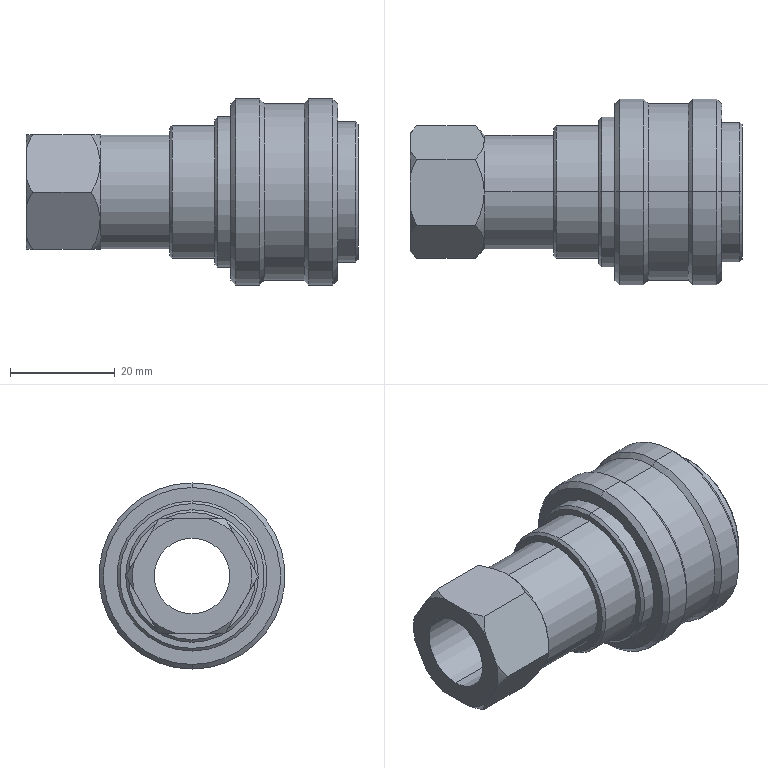Part | STEP file | 4-20.sldasm-Part-30 | 1 solid | 50 faces | box 63.246 x 35.458 x 35.458 mm | volume 27969 mm3 | cone 22 | cylinder 16 | plane 12 | commonest cylinder face diameters 35.458 x4 14.417 x2 21.692 x2 25.273 x2 26.67 x2 28.6 x2